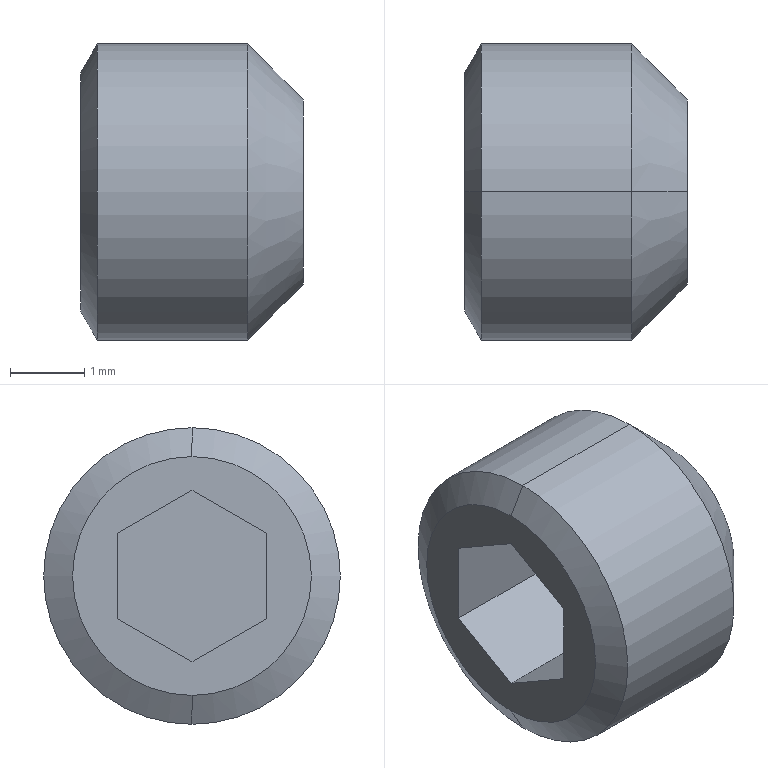Part | STEP file | socket set screw flat point_iso_ISO 4026 - M4 x 3-N | 1 solid | 15 faces | box 3 x 4 x 4 mm | volume 28.895 mm3 | plane 9 | cone 4 | cylinder 2 | commonest cylinder face diameters 4 x2
STEP:
#1=CARTESIAN_POINT('',(0.,0.,0.));
#2=DIRECTION('',(0.,0.,1.));
#3=DIRECTION('',(1.,0.,0.));
#4=AXIS2_PLACEMENT_3D('',#1,#2,#3);
#5=CARTESIAN_POINT('',(0.,0.,1.61));
#6=VERTEX_POINT('',#5);
#7=CARTESIAN_POINT('',(0.,0.,-1.61));
#8=VERTEX_POINT('',#7);
#9=CARTESIAN_POINT('',(0.,0.,0.));
#10=DIRECTION('',(-1.,0.,0.));
#11=DIRECTION('',(0.,0.,1.));
#12=AXIS2_PLACEMENT_3D('',#9,#10,#11);
#13=CIRCLE('',#12,1.61);
#14=CARTESIAN_POINT('',(0.,0.,0.));
#15=DIRECTION('',(1.,0.,0.));
#16=DIRECTION('',(0.,0.,-1.));
#17=AXIS2_PLACEMENT_3D('',#14,#15,#16);
#18=CONICAL_SURFACE('',#17,1.61,1.047);
#19=CARTESIAN_POINT('',(3.142,0.));
#20=DIRECTION('',(-1.,0.));
#21=VECTOR('',#20,1.);
#22=LINE('',#19,#21);
#23=(GEOMETRIC_REPRESENTATION_CONTEXT(2)PARAMETRIC_REPRESENTATION_CONTEXT()REPRESENTATION_CONTEXT('',''));
#24=DEFINITIONAL_REPRESENTATION('',(#22),#23);
#25=PCURVE('',#18,#24);
#26=CARTESIAN_POINT('',(0.,0.,0.));
#27=DIRECTION('',(-1.,0.,0.));
#28=DIRECTION('',(0.,0.,1.));
#29=AXIS2_PLACEMENT_3D('',#26,#27,#28);
#30=PLANE('',#29);
#31=CARTESIAN_POINT('',(0.,0.));
#32=DIRECTION('',(1.,0.));
#33=AXIS2_PLACEMENT_2D('',#31,#32);
#34=CIRCLE('',#33,1.61);
#35=(GEOMETRIC_REPRESENTATION_CONTEXT(2)PARAMETRIC_REPRESENTATION_CONTEXT()REPRESENTATION_CONTEXT('',''));
#36=DEFINITIONAL_REPRESENTATION('',(#34),#35);
#37=PCURVE('',#30,#36);
#38=SURFACE_CURVE('',#13,(#25,#37),.PCURVE_S1.);
#39=EDGE_CURVE('',#6,#8,#38,.T.);
#40=ORIENTED_EDGE('',*,*,#39,.F.);
#41=CARTESIAN_POINT('',(0.2252,0.,2.));
#42=VERTEX_POINT('',#41);
#43=CARTESIAN_POINT('',(0.,0.,1.61));
#44=DIRECTION('',(0.5,0.,0.866));
#45=VECTOR('',#44,1.);
#46=LINE('',#43,#45);
#47=CARTESIAN_POINT('',(3.142,0.));
#48=DIRECTION('',(0.,1.));
#49=VECTOR('',#48,1.);
#50=LINE('',#47,#49);
#51=(GEOMETRIC_REPRESENTATION_CONTEXT(2)PARAMETRIC_REPRESENTATION_CONTEXT()REPRESENTATION_CONTEXT('',''));
#52=DEFINITIONAL_REPRESENTATION('',(#50),#51);
#53=PCURVE('',#18,#52);
#54=CARTESIAN_POINT('',(0.,0.,0.));
#55=DIRECTION('',(1.,0.,0.));
#56=DIRECTION('',(0.,0.,-1.));
#57=AXIS2_PLACEMENT_3D('',#54,#55,#56);
#58=CONICAL_SURFACE('',#57,1.61,1.047);
#59=CARTESIAN_POINT('',(3.142,0.));
#60=DIRECTION('',(0.,1.));
#61=VECTOR('',#60,1.);
#62=LINE('',#59,#61);
#63=(GEOMETRIC_REPRESENTATION_CONTEXT(2)PARAMETRIC_REPRESENTATION_CONTEXT()REPRESENTATION_CONTEXT('',''));
#64=DEFINITIONAL_REPRESENTATION('',(#62),#63);
#65=PCURVE('',#58,#64);
#66=SURFACE_CURVE('',#46,(#53,#65),.PCURVE_S1.);
#67=EDGE_CURVE('',#6,#42,#66,.T.);
#68=ORIENTED_EDGE('',*,*,#67,.T.);
#69=CARTESIAN_POINT('',(0.2252,0.,-2.));
#70=VERTEX_POINT('',#69);
#71=CARTESIAN_POINT('',(0.2252,0.,0.));
#72=DIRECTION('',(-1.,0.,0.));
#73=DIRECTION('',(0.,0.,1.));
#74=AXIS2_PLACEMENT_3D('',#71,#72,#73);
#75=CIRCLE('',#74,2.);
#76=CARTESIAN_POINT('',(3.142,0.2252));
#77=DIRECTION('',(-1.,0.));
#78=VECTOR('',#77,1.);
#79=LINE('',#76,#78);
#80=(GEOMETRIC_REPRESENTATION_CONTEXT(2)PARAMETRIC_REPRESENTATION_CONTEXT()REPRESENTATION_CONTEXT('',''));
#81=DEFINITIONAL_REPRESENTATION('',(#79),#80);
#82=PCURVE('',#18,#81);
#83=CARTESIAN_POINT('',(-12.7,0.,0.));
#84=DIRECTION('',(-1.,0.,0.));
#85=DIRECTION('',(0.,0.,1.));
#86=AXIS2_PLACEMENT_3D('',#83,#84,#85);
#87=CYLINDRICAL_SURFACE('',#86,2.);
#88=CARTESIAN_POINT('',(0.,-12.925));
#89=DIRECTION('',(1.,0.));
#90=VECTOR('',#89,1.);
#91=LINE('',#88,#90);
#92=(GEOMETRIC_REPRESENTATION_CONTEXT(2)PARAMETRIC_REPRESENTATION_CONTEXT()REPRESENTATION_CONTEXT('',''));
#93=DEFINITIONAL_REPRESENTATION('',(#91),#92);
#94=PCURVE('',#87,#93);
#95=SURFACE_CURVE('',#75,(#82,#94),.PCURVE_S1.);
#96=EDGE_CURVE('',#42,#70,#95,.T.);
#97=ORIENTED_EDGE('',*,*,#96,.T.);
#98=CARTESIAN_POINT('',(0.,0.,-1.61));
#99=DIRECTION('',(0.5,0.,-0.866));
#100=VECTOR('',#99,1.);
#101=LINE('',#98,#100);
#102=CARTESIAN_POINT('',(0.,0.));
#103=DIRECTION('',(0.,1.));
#104=VECTOR('',#103,1.);
#105=LINE('',#102,#104);
#106=(GEOMETRIC_REPRESENTATION_CONTEXT(2)PARAMETRIC_REPRESENTATION_CONTEXT()REPRESENTATION_CONTEXT('',''));
#107=DEFINITIONAL_REPRESENTATION('',(#105),#106);
#108=PCURVE('',#18,#107);
#109=CARTESIAN_POINT('',(6.283,0.));
#110=DIRECTION('',(0.,1.));
#111=VECTOR('',#110,1.);
#112=LINE('',#109,#111);
#113=(GEOMETRIC_REPRESENTATION_CONTEXT(2)PARAMETRIC_REPRESENTATION_CONTEXT()REPRESENTATION_CONTEXT('',''));
#114=DEFINITIONAL_REPRESENTATION('',(#112),#113);
#115=PCURVE('',#58,#114);
#116=SURFACE_CURVE('',#101,(#108,#115),.PCURVE_S1.);
#117=EDGE_CURVE('',#8,#70,#116,.T.);
#118=ORIENTED_EDGE('',*,*,#117,.F.);
#119=EDGE_LOOP('',(#40,#68,#97,#118));
#120=FACE_BOUND('',#119,.T.);
#121=ADVANCED_FACE('',(#120),#18,.T.);
#122=CARTESIAN_POINT('',(2.25,0.,2.));
#123=VERTEX_POINT('',#122);
#124=CARTESIAN_POINT('',(2.25,0.,-2.));
#125=VERTEX_POINT('',#124);
#126=CARTESIAN_POINT('',(2.25,0.,0.));
#127=DIRECTION('',(-1.,0.,0.));
#128=DIRECTION('',(0.,0.,1.));
#129=AXIS2_PLACEMENT_3D('',#126,#127,#128);
#130=CIRCLE('',#129,2.);
#131=CARTESIAN_POINT('',(0.,-14.95));
#132=DIRECTION('',(1.,0.));
#133=VECTOR('',#132,1.);
#134=LINE('',#131,#133);
#135=(GEOMETRIC_REPRESENTATION_CONTEXT(2)PARAMETRIC_REPRESENTATION_CONTEXT()REPRESENTATION_CONTEXT('',''));
#136=DEFINITIONAL_REPRESENTATION('',(#134),#135);
#137=PCURVE('',#87,#136);
#138=CARTESIAN_POINT('',(2.25,0.,0.));
#139=DIRECTION('',(-1.,0.,0.));
#140=DIRECTION('',(0.,0.,1.));
#141=AXIS2_PLACEMENT_3D('',#138,#139,#140);
#142=CONICAL_SURFACE('',#141,2.,0.7854);
#143=CARTESIAN_POINT('',(0.,0.));
#144=DIRECTION('',(1.,0.));
#145=VECTOR('',#144,1.);
#146=LINE('',#143,#145);
#147=(GEOMETRIC_REPRESENTATION_CONTEXT(2)PARAMETRIC_REPRESENTATION_CONTEXT()REPRESENTATION_CONTEXT('',''));
#148=DEFINITIONAL_REPRESENTATION('',(#146),#147);
#149=PCURVE('',#142,#148);
#150=SURFACE_CURVE('',#130,(#137,#149),.PCURVE_S1.);
#151=EDGE_CURVE('',#123,#125,#150,.T.);
#152=ORIENTED_EDGE('',*,*,#151,.T.);
#153=CARTESIAN_POINT('',(-12.7,0.,-2.));
#154=DIRECTION('',(-1.,0.,0.));
#155=VECTOR('',#154,1.);
#156=LINE('',#153,#155);
#157=CARTESIAN_POINT('',(3.142,0.));
#158=DIRECTION('',(0.,1.));
#159=VECTOR('',#158,1.);
#160=LINE('',#157,#159);
#161=(GEOMETRIC_REPRESENTATION_CONTEXT(2)PARAMETRIC_REPRESENTATION_CONTEXT()REPRESENTATION_CONTEXT('',''));
#162=DEFINITIONAL_REPRESENTATION('',(#160),#161);
#163=PCURVE('',#87,#162);
#164=CARTESIAN_POINT('',(-12.7,0.,0.));
#165=DIRECTION('',(-1.,0.,0.));
#166=DIRECTION('',(0.,0.,1.));
#167=AXIS2_PLACEMENT_3D('',#164,#165,#166);
#168=CYLINDRICAL_SURFACE('',#167,2.);
#169=CARTESIAN_POINT('',(3.142,0.));
#170=DIRECTION('',(0.,1.));
#171=VECTOR('',#170,1.);
#172=LINE('',#169,#171);
#173=(GEOMETRIC_REPRESENTATION_CONTEXT(2)PARAMETRIC_REPRESENTATION_CONTEXT()REPRESENTATION_CONTEXT('',''));
#174=DEFINITIONAL_REPRESENTATION('',(#172),#173);
#175=PCURVE('',#168,#174);
#176=SURFACE_CURVE('',#156,(#163,#175),.PCURVE_S1.);
#177=EDGE_CURVE('',#125,#70,#176,.T.);
#178=ORIENTED_EDGE('',*,*,#177,.T.);
#179=ORIENTED_EDGE('',*,*,#96,.F.);
#180=CARTESIAN_POINT('',(-12.7,0.,2.));
#181=DIRECTION('',(-1.,0.,0.));
#182=VECTOR('',#181,1.);
#183=LINE('',#180,#182);
#184=CARTESIAN_POINT('',(0.,0.));
#185=DIRECTION('',(0.,1.));
#186=VECTOR('',#185,1.);
#187=LINE('',#184,#186);
#188=(GEOMETRIC_REPRESENTATION_CONTEXT(2)PARAMETRIC_REPRESENTATION_CONTEXT()REPRESENTATION_CONTEXT('',''));
#189=DEFINITIONAL_REPRESENTATION('',(#187),#188);
#190=PCURVE('',#87,#189);
#191=CARTESIAN_POINT('',(6.283,0.));
#192=DIRECTION('',(0.,1.));
#193=VECTOR('',#192,1.);
#194=LINE('',#191,#193);
#195=(GEOMETRIC_REPRESENTATION_CONTEXT(2)PARAMETRIC_REPRESENTATION_CONTEXT()REPRESENTATION_CONTEXT('',''));
#196=DEFINITIONAL_REPRESENTATION('',(#194),#195);
#197=PCURVE('',#168,#196);
#198=SURFACE_CURVE('',#183,(#190,#197),.PCURVE_S1.);
#199=EDGE_CURVE('',#123,#42,#198,.T.);
#200=ORIENTED_EDGE('',*,*,#199,.F.);
#201=EDGE_LOOP('',(#152,#178,#179,#200));
#202=FACE_BOUND('',#201,.T.);
#203=ADVANCED_FACE('',(#202),#87,.T.);
#204=CARTESIAN_POINT('',(3.,0.,1.25));
#205=VERTEX_POINT('',#204);
#206=CARTESIAN_POINT('',(3.,0.,-1.25));
#207=VERTEX_POINT('',#206);
#208=CARTESIAN_POINT('',(3.,0.,0.));
#209=DIRECTION('',(-1.,0.,0.));
#210=DIRECTION('',(0.,0.,1.));
#211=AXIS2_PLACEMENT_3D('',#208,#209,#210);
#212=CIRCLE('',#211,1.25);
#213=CARTESIAN_POINT('',(0.,-0.75));
#214=DIRECTION('',(1.,0.));
#215=VECTOR('',#214,1.);
#216=LINE('',#213,#215);
#217=(GEOMETRIC_REPRESENTATION_CONTEXT(2)PARAMETRIC_REPRESENTATION_CONTEXT()REPRESENTATION_CONTEXT('',''));
#218=DEFINITIONAL_REPRESENTATION('',(#216),#217);
#219=PCURVE('',#142,#218);
#220=CARTESIAN_POINT('',(3.,1.25,0.));
#221=DIRECTION('',(1.,0.,0.));
#222=DIRECTION('',(0.,0.,-1.));
#223=AXIS2_PLACEMENT_3D('',#220,#221,#222);
#224=PLANE('',#223);
#225=CARTESIAN_POINT('',(-1.25,-1.25));
#226=CARTESIAN_POINT('',(-1.25,0.9151));
#227=CARTESIAN_POINT('',(0.625,-0.1675));
#228=CARTESIAN_POINT('',(2.5,-1.25));
#229=CARTESIAN_POINT('',(0.625,-2.333));
#230=CARTESIAN_POINT('',(-1.25,-3.415));
#231=CARTESIAN_POINT('',(-1.25,-1.25));
#232=(BOUNDED_CURVE()B_SPLINE_CURVE(2,(#225,#226,#227,#228,#229,#230,#231),.UNSPECIFIED.,.T.,.F.)B_SPLINE_CURVE_WITH_KNOTS((1,2,2,2,2,1),(-2.094,0.,2.094,4.189,6.283,8.378),.UNSPECIFIED.)CURVE()GEOMETRIC_REPRESENTATION_ITEM()RATIONAL_B_SPLINE_CURVE((1.,0.5,1.,0.5,1.,0.5,1.))REPRESENTATION_ITEM(''));
#233=(GEOMETRIC_REPRESENTATION_CONTEXT(2)PARAMETRIC_REPRESENTATION_CONTEXT()REPRESENTATION_CONTEXT('',''));
#234=DEFINITIONAL_REPRESENTATION('',(#232),#233);
#235=PCURVE('',#224,#234);
#236=SURFACE_CURVE('',#212,(#219,#235),.PCURVE_S1.);
#237=EDGE_CURVE('',#205,#207,#236,.T.);
#238=ORIENTED_EDGE('',*,*,#237,.T.);
#239=CARTESIAN_POINT('',(2.25,0.,-2.));
#240=DIRECTION('',(-0.7071,0.,-0.7071));
#241=VECTOR('',#240,1.);
#242=LINE('',#239,#241);
#243=CARTESIAN_POINT('',(3.142,0.));
#244=DIRECTION('',(0.,1.));
#245=VECTOR('',#244,1.);
#246=LINE('',#243,#245);
#247=(GEOMETRIC_REPRESENTATION_CONTEXT(2)PARAMETRIC_REPRESENTATION_CONTEXT()REPRESENTATION_CONTEXT('',''));
#248=DEFINITIONAL_REPRESENTATION('',(#246),#247);
#249=PCURVE('',#142,#248);
#250=CARTESIAN_POINT('',(2.25,0.,0.));
#251=DIRECTION('',(-1.,0.,0.));
#252=DIRECTION('',(0.,0.,1.));
#253=AXIS2_PLACEMENT_3D('',#250,#251,#252);
#254=CONICAL_SURFACE('',#253,2.,0.7854);
#255=CARTESIAN_POINT('',(3.142,0.));
#256=DIRECTION('',(0.,1.));
#257=VECTOR('',#256,1.);
#258=LINE('',#255,#257);
#259=(GEOMETRIC_REPRESENTATION_CONTEXT(2)PARAMETRIC_REPRESENTATION_CONTEXT()REPRESENTATION_CONTEXT('',''));
#260=DEFINITIONAL_REPRESENTATION('',(#258),#259);
#261=PCURVE('',#254,#260);
#262=SURFACE_CURVE('',#242,(#249,#261),.PCURVE_S1.);
#263=EDGE_CURVE('',#207,#125,#262,.T.);
#264=ORIENTED_EDGE('',*,*,#263,.T.);
#265=ORIENTED_EDGE('',*,*,#151,.F.);
#266=CARTESIAN_POINT('',(2.25,0.,2.));
#267=DIRECTION('',(-0.7071,0.,0.7071));
#268=VECTOR('',#267,1.);
#269=LINE('',#266,#268);
#270=CARTESIAN_POINT('',(0.,0.));
#271=DIRECTION('',(0.,1.));
#272=VECTOR('',#271,1.);
#273=LINE('',#270,#272);
#274=(GEOMETRIC_REPRESENTATION_CONTEXT(2)PARAMETRIC_REPRESENTATION_CONTEXT()REPRESENTATION_CONTEXT('',''));
#275=DEFINITIONAL_REPRESENTATION('',(#273),#274);
#276=PCURVE('',#142,#275);
#277=CARTESIAN_POINT('',(6.283,0.));
#278=DIRECTION('',(0.,1.));
#279=VECTOR('',#278,1.);
#280=LINE('',#277,#279);
#281=(GEOMETRIC_REPRESENTATION_CONTEXT(2)PARAMETRIC_REPRESENTATION_CONTEXT()REPRESENTATION_CONTEXT('',''));
#282=DEFINITIONAL_REPRESENTATION('',(#280),#281);
#283=PCURVE('',#254,#282);
#284=SURFACE_CURVE('',#269,(#276,#283),.PCURVE_S1.);
#285=EDGE_CURVE('',#205,#123,#284,.T.);
#286=ORIENTED_EDGE('',*,*,#285,.F.);
#287=EDGE_LOOP('',(#238,#264,#265,#286));
#288=FACE_BOUND('',#287,.T.);
#289=ADVANCED_FACE('',(#288),#142,.T.);
#290=CARTESIAN_POINT('',(0.,0.,0.));
#291=DIRECTION('',(-1.,0.,0.));
#292=DIRECTION('',(0.,0.,1.));
#293=AXIS2_PLACEMENT_3D('',#290,#291,#292);
#294=CIRCLE('',#293,1.61);
#295=CARTESIAN_POINT('',(0.,0.));
#296=DIRECTION('',(1.,0.));
#297=AXIS2_PLACEMENT_2D('',#295,#296);
#298=CIRCLE('',#297,1.61);
#299=(GEOMETRIC_REPRESENTATION_CONTEXT(2)PARAMETRIC_REPRESENTATION_CONTEXT()REPRESENTATION_CONTEXT('',''));
#300=DEFINITIONAL_REPRESENTATION('',(#298),#299);
#301=PCURVE('',#30,#300);
#302=CARTESIAN_POINT('',(9.425,0.));
#303=DIRECTION('',(-1.,0.));
#304=VECTOR('',#303,1.);
#305=LINE('',#302,#304);
#306=(GEOMETRIC_REPRESENTATION_CONTEXT(2)PARAMETRIC_REPRESENTATION_CONTEXT()REPRESENTATION_CONTEXT('',''));
#307=DEFINITIONAL_REPRESENTATION('',(#305),#306);
#308=PCURVE('',#58,#307);
#309=SURFACE_CURVE('',#294,(#301,#308),.PCURVE_S1.);
#310=EDGE_CURVE('',#8,#6,#309,.T.);
#311=ORIENTED_EDGE('',*,*,#310,.T.);
#312=ORIENTED_EDGE('',*,*,#39,.T.);
#313=EDGE_LOOP('',(#311,#312));
#314=FACE_BOUND('',#313,.T.);
#315=CARTESIAN_POINT('',(0.,1.,0.5774));
#316=VERTEX_POINT('',#315);
#317=CARTESIAN_POINT('',(0.,1.,-0.5774));
#318=VERTEX_POINT('',#317);
#319=CARTESIAN_POINT('',(0.,1.,0.5774));
#320=DIRECTION('',(0.,0.,-1.));
#321=VECTOR('',#320,1.);
#322=LINE('',#319,#321);
#323=CARTESIAN_POINT('',(0.5774,1.));
#324=DIRECTION('',(-1.,0.));
#325=VECTOR('',#324,1.);
#326=LINE('',#323,#325);
#327=(GEOMETRIC_REPRESENTATION_CONTEXT(2)PARAMETRIC_REPRESENTATION_CONTEXT()REPRESENTATION_CONTEXT('',''));
#328=DEFINITIONAL_REPRESENTATION('',(#326),#327);
#329=PCURVE('',#30,#328);
#330=CARTESIAN_POINT('',(1.5,1.,0.5774));
#331=DIRECTION('',(0.,1.,0.));
#332=DIRECTION('',(0.,0.,1.));
#333=AXIS2_PLACEMENT_3D('',#330,#331,#332);
#334=PLANE('',#333);
#335=CARTESIAN_POINT('',(0.,-1.5));
#336=DIRECTION('',(-1.,0.));
#337=VECTOR('',#336,1.);
#338=LINE('',#335,#337);
#339=(GEOMETRIC_REPRESENTATION_CONTEXT(2)PARAMETRIC_REPRESENTATION_CONTEXT()REPRESENTATION_CONTEXT('',''));
#340=DEFINITIONAL_REPRESENTATION('',(#338),#339);
#341=PCURVE('',#334,#340);
#342=SURFACE_CURVE('',#322,(#329,#341),.PCURVE_S1.);
#343=EDGE_CURVE('',#316,#318,#342,.T.);
#344=ORIENTED_EDGE('',*,*,#343,.F.);
#345=CARTESIAN_POINT('',(0.,0.,1.155));
#346=VERTEX_POINT('',#345);
#347=CARTESIAN_POINT('',(0.,1.,0.5774));
#348=DIRECTION('',(0.,-0.866,0.5));
#349=VECTOR('',#348,1.);
#350=LINE('',#347,#349);
#351=CARTESIAN_POINT('',(0.5774,1.));
#352=DIRECTION('',(0.5,-0.866));
#353=VECTOR('',#352,1.);
#354=LINE('',#351,#353);
#355=(GEOMETRIC_REPRESENTATION_CONTEXT(2)PARAMETRIC_REPRESENTATION_CONTEXT()REPRESENTATION_CONTEXT('',''));
#356=DEFINITIONAL_REPRESENTATION('',(#354),#355);
#357=PCURVE('',#30,#356);
#358=CARTESIAN_POINT('',(1.5,1.,0.5774));
#359=DIRECTION('',(0.,-0.5,-0.866));
#360=DIRECTION('',(0.,0.866,-0.5));
#361=AXIS2_PLACEMENT_3D('',#358,#359,#360);
#362=PLANE('',#361);
#363=CARTESIAN_POINT('',(0.,-1.5));
#364=DIRECTION('',(-1.,0.));
#365=VECTOR('',#364,1.);
#366=LINE('',#363,#365);
#367=(GEOMETRIC_REPRESENTATION_CONTEXT(2)PARAMETRIC_REPRESENTATION_CONTEXT()REPRESENTATION_CONTEXT('',''));
#368=DEFINITIONAL_REPRESENTATION('',(#366),#367);
#369=PCURVE('',#362,#368);
#370=SURFACE_CURVE('',#350,(#357,#369),.PCURVE_S1.);
#371=EDGE_CURVE('',#316,#346,#370,.T.);
#372=ORIENTED_EDGE('',*,*,#371,.T.);
#373=CARTESIAN_POINT('',(0.,-1.,0.5774));
#374=VERTEX_POINT('',#373);
#375=CARTESIAN_POINT('',(0.,-1.,0.5774));
#376=DIRECTION('',(0.,0.866,0.5));
#377=VECTOR('',#376,1.);
#378=LINE('',#375,#377);
#379=CARTESIAN_POINT('',(0.5774,-1.));
#380=DIRECTION('',(0.5,0.866));
#381=VECTOR('',#380,1.);
#382=LINE('',#379,#381);
#383=(GEOMETRIC_REPRESENTATION_CONTEXT(2)PARAMETRIC_REPRESENTATION_CONTEXT()REPRESENTATION_CONTEXT('',''));
#384=DEFINITIONAL_REPRESENTATION('',(#382),#383);
#385=PCURVE('',#30,#384);
#386=CARTESIAN_POINT('',(1.5,-1.,0.5774));
#387=DIRECTION('',(0.,-0.5,0.866));
#388=DIRECTION('',(0.,-0.866,-0.5));
#389=AXIS2_PLACEMENT_3D('',#386,#387,#388);
#390=PLANE('',#389);
#391=CARTESIAN_POINT('',(0.,-1.5));
#392=DIRECTION('',(-1.,0.));
#393=VECTOR('',#392,1.);
#394=LINE('',#391,#393);
#395=(GEOMETRIC_REPRESENTATION_CONTEXT(2)PARAMETRIC_REPRESENTATION_CONTEXT()REPRESENTATION_CONTEXT('',''));
#396=DEFINITIONAL_REPRESENTATION('',(#394),#395);
#397=PCURVE('',#390,#396);
#398=SURFACE_CURVE('',#378,(#385,#397),.PCURVE_S1.);
#399=EDGE_CURVE('',#374,#346,#398,.T.);
#400=ORIENTED_EDGE('',*,*,#399,.F.);
#401=CARTESIAN_POINT('',(0.,-1.,-0.5774));
#402=VERTEX_POINT('',#401);
#403=CARTESIAN_POINT('',(0.,-1.,0.5774));
#404=DIRECTION('',(0.,0.,-1.));
#405=VECTOR('',#404,1.);
#406=LINE('',#403,#405);
#407=CARTESIAN_POINT('',(0.5774,-1.));
#408=DIRECTION('',(-1.,0.));
#409=VECTOR('',#408,1.);
#410=LINE('',#407,#409);
#411=(GEOMETRIC_REPRESENTATION_CONTEXT(2)PARAMETRIC_REPRESENTATION_CONTEXT()REPRESENTATION_CONTEXT('',''));
#412=DEFINITIONAL_REPRESENTATION('',(#410),#411);
#413=PCURVE('',#30,#412);
#414=CARTESIAN_POINT('',(1.5,-1.,0.5774));
#415=DIRECTION('',(0.,1.,0.));
#416=DIRECTION('',(0.,0.,1.));
#417=AXIS2_PLACEMENT_3D('',#414,#415,#416);
#418=PLANE('',#417);
#419=CARTESIAN_POINT('',(0.,-1.5));
#420=DIRECTION('',(-1.,0.));
#421=VECTOR('',#420,1.);
#422=LINE('',#419,#421);
#423=(GEOMETRIC_REPRESENTATION_CONTEXT(2)PARAMETRIC_REPRESENTATION_CONTEXT()REPRESENTATION_CONTEXT('',''));
#424=DEFINITIONAL_REPRESENTATION('',(#422),#423);
#425=PCURVE('',#418,#424);
#426=SURFACE_CURVE('',#406,(#413,#425),.PCURVE_S1.);
#427=EDGE_CURVE('',#374,#402,#426,.T.);
#428=ORIENTED_EDGE('',*,*,#427,.T.);
#429=CARTESIAN_POINT('',(0.,0.,-1.155));
#430=VERTEX_POINT('',#429);
#431=CARTESIAN_POINT('',(0.,-1.,-0.5774));
#432=DIRECTION('',(0.,0.866,-0.5));
#433=VECTOR('',#432,1.);
#434=LINE('',#431,#433);
#435=CARTESIAN_POINT('',(-0.5774,-1.));
#436=DIRECTION('',(-0.5,0.866));
#437=VECTOR('',#436,1.);
#438=LINE('',#435,#437);
#439=(GEOMETRIC_REPRESENTATION_CONTEXT(2)PARAMETRIC_REPRESENTATION_CONTEXT()REPRESENTATION_CONTEXT('',''));
#440=DEFINITIONAL_REPRESENTATION('',(#438),#439);
#441=PCURVE('',#30,#440);
#442=CARTESIAN_POINT('',(1.5,-1.,-0.5774));
#443=DIRECTION('',(0.,0.5,0.866));
#444=DIRECTION('',(0.,-0.866,0.5));
#445=AXIS2_PLACEMENT_3D('',#442,#443,#444);
#446=PLANE('',#445);
#447=CARTESIAN_POINT('',(0.,-1.5));
#448=DIRECTION('',(-1.,0.));
#449=VECTOR('',#448,1.);
#450=LINE('',#447,#449);
#451=(GEOMETRIC_REPRESENTATION_CONTEXT(2)PARAMETRIC_REPRESENTATION_CONTEXT()REPRESENTATION_CONTEXT('',''));
#452=DEFINITIONAL_REPRESENTATION('',(#450),#451);
#453=PCURVE('',#446,#452);
#454=SURFACE_CURVE('',#434,(#441,#453),.PCURVE_S1.);
#455=EDGE_CURVE('',#402,#430,#454,.T.);
#456=ORIENTED_EDGE('',*,*,#455,.T.);
#457=CARTESIAN_POINT('',(0.,1.,-0.5774));
#458=DIRECTION('',(0.,-0.866,-0.5));
#459=VECTOR('',#458,1.);
#460=LINE('',#457,#459);
#461=CARTESIAN_POINT('',(-0.5774,1.));
#462=DIRECTION('',(-0.5,-0.866));
#463=VECTOR('',#462,1.);
#464=LINE('',#461,#463);
#465=(GEOMETRIC_REPRESENTATION_CONTEXT(2)PARAMETRIC_REPRESENTATION_CONTEXT()REPRESENTATION_CONTEXT('',''));
#466=DEFINITIONAL_REPRESENTATION('',(#464),#465);
#467=PCURVE('',#30,#466);
#468=CARTESIAN_POINT('',(1.5,1.,-0.5774));
#469=DIRECTION('',(0.,0.5,-0.866));
#470=DIRECTION('',(0.,0.866,0.5));
#471=AXIS2_PLACEMENT_3D('',#468,#469,#470);
#472=PLANE('',#471);
#473=CARTESIAN_POINT('',(0.,-1.5));
#474=DIRECTION('',(-1.,0.));
#475=VECTOR('',#474,1.);
#476=LINE('',#473,#475);
#477=(GEOMETRIC_REPRESENTATION_CONTEXT(2)PARAMETRIC_REPRESENTATION_CONTEXT()REPRESENTATION_CONTEXT('',''));
#478=DEFINITIONAL_REPRESENTATION('',(#476),#477);
#479=PCURVE('',#472,#478);
#480=SURFACE_CURVE('',#460,(#467,#479),.PCURVE_S1.);
#481=EDGE_CURVE('',#318,#430,#480,.T.);
#482=ORIENTED_EDGE('',*,*,#481,.F.);
#483=EDGE_LOOP('',(#344,#372,#400,#428,#456,#482));
#484=FACE_BOUND('',#483,.T.);
#485=ADVANCED_FACE('',(#314,#484),#30,.T.);
#486=ORIENTED_EDGE('',*,*,#237,.F.);
#487=CARTESIAN_POINT('',(3.,0.,0.));
#488=DIRECTION('',(-1.,0.,0.));
#489=DIRECTION('',(0.,0.,1.));
#490=AXIS2_PLACEMENT_3D('',#487,#488,#489);
#491=CIRCLE('',#490,1.25);
#492=CARTESIAN_POINT('',(-1.25,-1.25));
#493=CARTESIAN_POINT('',(-1.25,0.9151));
#494=CARTESIAN_POINT('',(0.625,-0.1675));
#495=CARTESIAN_POINT('',(2.5,-1.25));
#496=CARTESIAN_POINT('',(0.625,-2.333));
#497=CARTESIAN_POINT('',(-1.25,-3.415));
#498=CARTESIAN_POINT('',(-1.25,-1.25));
#499=(BOUNDED_CURVE()B_SPLINE_CURVE(2,(#492,#493,#494,#495,#496,#497,#498),.UNSPECIFIED.,.T.,.F.)B_SPLINE_CURVE_WITH_KNOTS((1,2,2,2,2,1),(-2.094,0.,2.094,4.189,6.283,8.378),.UNSPECIFIED.)CURVE()GEOMETRIC_REPRESENTATION_ITEM()RATIONAL_B_SPLINE_CURVE((1.,0.5,1.,0.5,1.,0.5,1.))REPRESENTATION_ITEM(''));
#500=(GEOMETRIC_REPRESENTATION_CONTEXT(2)PARAMETRIC_REPRESENTATION_CONTEXT()REPRESENTATION_CONTEXT('',''));
#501=DEFINITIONAL_REPRESENTATION('',(#499),#500);
#502=PCURVE('',#224,#501);
#503=CARTESIAN_POINT('',(0.,-0.75));
#504=DIRECTION('',(1.,0.));
#505=VECTOR('',#504,1.);
#506=LINE('',#503,#505);
#507=(GEOMETRIC_REPRESENTATION_CONTEXT(2)PARAMETRIC_REPRESENTATION_CONTEXT()REPRESENTATION_CONTEXT('',''));
#508=DEFINITIONAL_REPRESENTATION('',(#506),#507);
#509=PCURVE('',#254,#508);
#510=SURFACE_CURVE('',#491,(#502,#509),.PCURVE_S1.);
#511=EDGE_CURVE('',#207,#205,#510,.T.);
#512=ORIENTED_EDGE('',*,*,#511,.F.);
#513=EDGE_LOOP('',(#486,#512));
#514=FACE_BOUND('',#513,.T.);
#515=ADVANCED_FACE('',(#514),#224,.T.);
#516=ORIENTED_EDGE('',*,*,#263,.F.);
#517=ORIENTED_EDGE('',*,*,#511,.T.);
#518=ORIENTED_EDGE('',*,*,#285,.T.);
#519=CARTESIAN_POINT('',(2.25,0.,0.));
#520=DIRECTION('',(-1.,0.,0.));
#521=DIRECTION('',(0.,0.,1.));
#522=AXIS2_PLACEMENT_3D('',#519,#520,#521);
#523=CIRCLE('',#522,2.);
#524=CARTESIAN_POINT('',(0.,0.));
#525=DIRECTION('',(1.,0.));
#526=VECTOR('',#525,1.);
#527=LINE('',#524,#526);
#528=(GEOMETRIC_REPRESENTATION_CONTEXT(2)PARAMETRIC_REPRESENTATION_CONTEXT()REPRESENTATION_CONTEXT('',''));
#529=DEFINITIONAL_REPRESENTATION('',(#527),#528);
#530=PCURVE('',#254,#529);
#531=CARTESIAN_POINT('',(0.,-14.95));
#532=DIRECTION('',(1.,0.));
#533=VECTOR('',#532,1.);
#534=LINE('',#531,#533);
#535=(GEOMETRIC_REPRESENTATION_CONTEXT(2)PARAMETRIC_REPRESENTATION_CONTEXT()REPRESENTATION_CONTEXT('',''));
#536=DEFINITIONAL_REPRESENTATION('',(#534),#535);
#537=PCURVE('',#168,#536);
#538=SURFACE_CURVE('',#523,(#530,#537),.PCURVE_S1.);
#539=EDGE_CURVE('',#125,#123,#538,.T.);
#540=ORIENTED_EDGE('',*,*,#539,.F.);
#541=EDGE_LOOP('',(#516,#517,#518,#540));
#542=FACE_BOUND('',#541,.T.);
#543=ADVANCED_FACE('',(#542),#254,.T.);
#544=ORIENTED_EDGE('',*,*,#177,.F.);
#545=ORIENTED_EDGE('',*,*,#539,.T.);
#546=ORIENTED_EDGE('',*,*,#199,.T.);
#547=CARTESIAN_POINT('',(0.2252,0.,0.));
#548=DIRECTION('',(-1.,0.,0.));
#549=DIRECTION('',(0.,0.,1.));
#550=AXIS2_PLACEMENT_3D('',#547,#548,#549);
#551=CIRCLE('',#550,2.);
#552=CARTESIAN_POINT('',(0.,-12.925));
#553=DIRECTION('',(1.,0.));
#554=VECTOR('',#553,1.);
#555=LINE('',#552,#554);
#556=(GEOMETRIC_REPRESENTATION_CONTEXT(2)PARAMETRIC_REPRESENTATION_CONTEXT()REPRESENTATION_CONTEXT('',''));
#557=DEFINITIONAL_REPRESENTATION('',(#555),#556);
#558=PCURVE('',#168,#557);
#559=CARTESIAN_POINT('',(9.425,0.2252));
#560=DIRECTION('',(-1.,0.));
#561=VECTOR('',#560,1.);
#562=LINE('',#559,#561);
#563=(GEOMETRIC_REPRESENTATION_CONTEXT(2)PARAMETRIC_REPRESENTATION_CONTEXT()REPRESENTATION_CONTEXT('',''));
#564=DEFINITIONAL_REPRESENTATION('',(#562),#563);
#565=PCURVE('',#58,#564);
#566=SURFACE_CURVE('',#551,(#558,#565),.PCURVE_S1.);
#567=EDGE_CURVE('',#70,#42,#566,.T.);
#568=ORIENTED_EDGE('',*,*,#567,.F.);
#569=EDGE_LOOP('',(#544,#545,#546,#568));
#570=FACE_BOUND('',#569,.T.);
#571=ADVANCED_FACE('',(#570),#168,.T.);
#572=ORIENTED_EDGE('',*,*,#67,.F.);
#573=ORIENTED_EDGE('',*,*,#310,.F.);
#574=ORIENTED_EDGE('',*,*,#117,.T.);
#575=ORIENTED_EDGE('',*,*,#567,.T.);
#576=EDGE_LOOP('',(#572,#573,#574,#575));
#577=FACE_BOUND('',#576,.T.);
#578=ADVANCED_FACE('',(#577),#58,.T.);
#579=ORIENTED_EDGE('',*,*,#371,.F.);
#580=CARTESIAN_POINT('',(1.5,1.,0.5774));
#581=VERTEX_POINT('',#580);
#582=CARTESIAN_POINT('',(1.5,1.,0.5774));
#583=DIRECTION('',(-1.,0.,0.));
#584=VECTOR('',#583,1.);
#585=LINE('',#582,#584);
#586=CARTESIAN_POINT('',(0.,0.));
#587=DIRECTION('',(0.,-1.));
#588=VECTOR('',#587,1.);
#589=LINE('',#586,#588);
#590=(GEOMETRIC_REPRESENTATION_CONTEXT(2)PARAMETRIC_REPRESENTATION_CONTEXT()REPRESENTATION_CONTEXT('',''));
#591=DEFINITIONAL_REPRESENTATION('',(#589),#590);
#592=PCURVE('',#362,#591);
#593=CARTESIAN_POINT('',(0.,0.));
#594=DIRECTION('',(0.,-1.));
#595=VECTOR('',#594,1.);
#596=LINE('',#593,#595);
#597=(GEOMETRIC_REPRESENTATION_CONTEXT(2)PARAMETRIC_REPRESENTATION_CONTEXT()REPRESENTATION_CONTEXT('',''));
#598=DEFINITIONAL_REPRESENTATION('',(#596),#597);
#599=PCURVE('',#334,#598);
#600=SURFACE_CURVE('',#585,(#592,#599),.PCURVE_S1.);
#601=EDGE_CURVE('',#581,#316,#600,.T.);
#602=ORIENTED_EDGE('',*,*,#601,.F.);
#603=CARTESIAN_POINT('',(1.5,0.,1.155));
#604=VERTEX_POINT('',#603);
#605=CARTESIAN_POINT('',(1.5,1.,0.5774));
#606=DIRECTION('',(0.,-0.866,0.5));
#607=VECTOR('',#606,1.);
#608=LINE('',#605,#607);
#609=CARTESIAN_POINT('',(0.,0.));
#610=DIRECTION('',(-1.,0.));
#611=VECTOR('',#610,1.);
#612=LINE('',#609,#611);
#613=(GEOMETRIC_REPRESENTATION_CONTEXT(2)PARAMETRIC_REPRESENTATION_CONTEXT()REPRESENTATION_CONTEXT('',''));
#614=DEFINITIONAL_REPRESENTATION('',(#612),#613);
#615=PCURVE('',#362,#614);
#616=CARTESIAN_POINT('',(1.5,0.,1.155));
#617=DIRECTION('',(-1.,0.,0.));
#618=DIRECTION('',(0.,0.,1.));
#619=AXIS2_PLACEMENT_3D('',#616,#617,#618);
#620=PLANE('',#619);
#621=CARTESIAN_POINT('',(-0.5774,1.));
#622=DIRECTION('',(0.5,-0.866));
#623=VECTOR('',#622,1.);
#624=LINE('',#621,#623);
#625=(GEOMETRIC_REPRESENTATION_CONTEXT(2)PARAMETRIC_REPRESENTATION_CONTEXT()REPRESENTATION_CONTEXT('',''));
#626=DEFINITIONAL_REPRESENTATION('',(#624),#625);
#627=PCURVE('',#620,#626);
#628=SURFACE_CURVE('',#608,(#615,#627),.PCURVE_S1.);
#629=EDGE_CURVE('',#581,#604,#628,.T.);
#630=ORIENTED_EDGE('',*,*,#629,.T.);
#631=CARTESIAN_POINT('',(1.5,0.,1.155));
#632=DIRECTION('',(-1.,0.,0.));
#633=VECTOR('',#632,1.);
#634=LINE('',#631,#633);
#635=CARTESIAN_POINT('',(-1.155,0.));
#636=DIRECTION('',(0.,-1.));
#637=VECTOR('',#636,1.);
#638=LINE('',#635,#637);
#639=(GEOMETRIC_REPRESENTATION_CONTEXT(2)PARAMETRIC_REPRESENTATION_CONTEXT()REPRESENTATION_CONTEXT('',''));
#640=DEFINITIONAL_REPRESENTATION('',(#638),#639);
#641=PCURVE('',#362,#640);
#642=CARTESIAN_POINT('',(-1.155,0.));
#643=DIRECTION('',(0.,-1.));
#644=VECTOR('',#643,1.);
#645=LINE('',#642,#644);
#646=(GEOMETRIC_REPRESENTATION_CONTEXT(2)PARAMETRIC_REPRESENTATION_CONTEXT()REPRESENTATION_CONTEXT('',''));
#647=DEFINITIONAL_REPRESENTATION('',(#645),#646);
#648=PCURVE('',#390,#647);
#649=SURFACE_CURVE('',#634,(#641,#648),.PCURVE_S1.);
#650=EDGE_CURVE('',#604,#346,#649,.T.);
#651=ORIENTED_EDGE('',*,*,#650,.T.);
#652=EDGE_LOOP('',(#579,#602,#630,#651));
#653=FACE_BOUND('',#652,.T.);
#654=ADVANCED_FACE('',(#653),#362,.T.);
#655=ORIENTED_EDGE('',*,*,#399,.T.);
#656=ORIENTED_EDGE('',*,*,#650,.F.);
#657=CARTESIAN_POINT('',(1.5,-1.,0.5774));
#658=VERTEX_POINT('',#657);
#659=CARTESIAN_POINT('',(1.5,-1.,0.5774));
#660=DIRECTION('',(0.,0.866,0.5));
#661=VECTOR('',#660,1.);
#662=LINE('',#659,#661);
#663=CARTESIAN_POINT('',(0.,0.));
#664=DIRECTION('',(-1.,0.));
#665=VECTOR('',#664,1.);
#666=LINE('',#663,#665);
#667=(GEOMETRIC_REPRESENTATION_CONTEXT(2)PARAMETRIC_REPRESENTATION_CONTEXT()REPRESENTATION_CONTEXT('',''));
#668=DEFINITIONAL_REPRESENTATION('',(#666),#667);
#669=PCURVE('',#390,#668);
#670=CARTESIAN_POINT('',(-0.5774,-1.));
#671=DIRECTION('',(0.5,0.866));
#672=VECTOR('',#671,1.);
#673=LINE('',#670,#672);
#674=(GEOMETRIC_REPRESENTATION_CONTEXT(2)PARAMETRIC_REPRESENTATION_CONTEXT()REPRESENTATION_CONTEXT('',''));
#675=DEFINITIONAL_REPRESENTATION('',(#673),#674);
#676=PCURVE('',#620,#675);
#677=SURFACE_CURVE('',#662,(#669,#676),.PCURVE_S1.);
#678=EDGE_CURVE('',#658,#604,#677,.T.);
#679=ORIENTED_EDGE('',*,*,#678,.F.);
#680=CARTESIAN_POINT('',(1.5,-1.,0.5774));
#681=DIRECTION('',(-1.,0.,0.));
#682=VECTOR('',#681,1.);
#683=LINE('',#680,#682);
#684=CARTESIAN_POINT('',(0.,0.));
#685=DIRECTION('',(0.,-1.));
#686=VECTOR('',#685,1.);
#687=LINE('',#684,#686);
#688=(GEOMETRIC_REPRESENTATION_CONTEXT(2)PARAMETRIC_REPRESENTATION_CONTEXT()REPRESENTATION_CONTEXT('',''));
#689=DEFINITIONAL_REPRESENTATION('',(#687),#688);
#690=PCURVE('',#390,#689);
#691=CARTESIAN_POINT('',(0.,0.));
#692=DIRECTION('',(0.,-1.));
#693=VECTOR('',#692,1.);
#694=LINE('',#691,#693);
#695=(GEOMETRIC_REPRESENTATION_CONTEXT(2)PARAMETRIC_REPRESENTATION_CONTEXT()REPRESENTATION_CONTEXT('',''));
#696=DEFINITIONAL_REPRESENTATION('',(#694),#695);
#697=PCURVE('',#418,#696);
#698=SURFACE_CURVE('',#683,(#690,#697),.PCURVE_S1.);
#699=EDGE_CURVE('',#658,#374,#698,.T.);
#700=ORIENTED_EDGE('',*,*,#699,.T.);
#701=EDGE_LOOP('',(#655,#656,#679,#700));
#702=FACE_BOUND('',#701,.T.);
#703=ADVANCED_FACE('',(#702),#390,.F.);
#704=ORIENTED_EDGE('',*,*,#427,.F.);
#705=ORIENTED_EDGE('',*,*,#699,.F.);
#706=CARTESIAN_POINT('',(1.5,-1.,-0.5774));
#707=VERTEX_POINT('',#706);
#708=CARTESIAN_POINT('',(1.5,-1.,0.5774));
#709=DIRECTION('',(0.,0.,-1.));
#710=VECTOR('',#709,1.);
#711=LINE('',#708,#710);
#712=CARTESIAN_POINT('',(0.,0.));
#713=DIRECTION('',(-1.,0.));
#714=VECTOR('',#713,1.);
#715=LINE('',#712,#714);
#716=(GEOMETRIC_REPRESENTATION_CONTEXT(2)PARAMETRIC_REPRESENTATION_CONTEXT()REPRESENTATION_CONTEXT('',''));
#717=DEFINITIONAL_REPRESENTATION('',(#715),#716);
#718=PCURVE('',#418,#717);
#719=CARTESIAN_POINT('',(-0.5774,-1.));
#720=DIRECTION('',(-1.,0.));
#721=VECTOR('',#720,1.);
#722=LINE('',#719,#721);
#723=(GEOMETRIC_REPRESENTATION_CONTEXT(2)PARAMETRIC_REPRESENTATION_CONTEXT()REPRESENTATION_CONTEXT('',''));
#724=DEFINITIONAL_REPRESENTATION('',(#722),#723);
#725=PCURVE('',#620,#724);
#726=SURFACE_CURVE('',#711,(#718,#725),.PCURVE_S1.);
#727=EDGE_CURVE('',#658,#707,#726,.T.);
#728=ORIENTED_EDGE('',*,*,#727,.T.);
#729=CARTESIAN_POINT('',(1.5,-1.,-0.5774));
#730=DIRECTION('',(-1.,0.,0.));
#731=VECTOR('',#730,1.);
#732=LINE('',#729,#731);
#733=CARTESIAN_POINT('',(-1.155,0.));
#734=DIRECTION('',(0.,-1.));
#735=VECTOR('',#734,1.);
#736=LINE('',#733,#735);
#737=(GEOMETRIC_REPRESENTATION_CONTEXT(2)PARAMETRIC_REPRESENTATION_CONTEXT()REPRESENTATION_CONTEXT('',''));
#738=DEFINITIONAL_REPRESENTATION('',(#736),#737);
#739=PCURVE('',#418,#738);
#740=CARTESIAN_POINT('',(0.,0.));
#741=DIRECTION('',(0.,-1.));
#742=VECTOR('',#741,1.);
#743=LINE('',#740,#742);
#744=(GEOMETRIC_REPRESENTATION_CONTEXT(2)PARAMETRIC_REPRESENTATION_CONTEXT()REPRESENTATION_CONTEXT('',''));
#745=DEFINITIONAL_REPRESENTATION('',(#743),#744);
#746=PCURVE('',#446,#745);
#747=SURFACE_CURVE('',#732,(#739,#746),.PCURVE_S1.);
#748=EDGE_CURVE('',#707,#402,#747,.T.);
#749=ORIENTED_EDGE('',*,*,#748,.T.);
#750=EDGE_LOOP('',(#704,#705,#728,#749));
#751=FACE_BOUND('',#750,.T.);
#752=ADVANCED_FACE('',(#751),#418,.T.);
#753=ORIENTED_EDGE('',*,*,#455,.F.);
#754=ORIENTED_EDGE('',*,*,#748,.F.);
#755=CARTESIAN_POINT('',(1.5,0.,-1.155));
#756=VERTEX_POINT('',#755);
#757=CARTESIAN_POINT('',(1.5,-1.,-0.5774));
#758=DIRECTION('',(0.,0.866,-0.5));
#759=VECTOR('',#758,1.);
#760=LINE('',#757,#759);
#761=CARTESIAN_POINT('',(0.,0.));
#762=DIRECTION('',(-1.,0.));
#763=VECTOR('',#762,1.);
#764=LINE('',#761,#763);
#765=(GEOMETRIC_REPRESENTATION_CONTEXT(2)PARAMETRIC_REPRESENTATION_CONTEXT()REPRESENTATION_CONTEXT('',''));
#766=DEFINITIONAL_REPRESENTATION('',(#764),#765);
#767=PCURVE('',#446,#766);
#768=CARTESIAN_POINT('',(-1.732,-1.));
#769=DIRECTION('',(-0.5,0.866));
#770=VECTOR('',#769,1.);
#771=LINE('',#768,#770);
#772=(GEOMETRIC_REPRESENTATION_CONTEXT(2)PARAMETRIC_REPRESENTATION_CONTEXT()REPRESENTATION_CONTEXT('',''));
#773=DEFINITIONAL_REPRESENTATION('',(#771),#772);
#774=PCURVE('',#620,#773);
#775=SURFACE_CURVE('',#760,(#767,#774),.PCURVE_S1.);
#776=EDGE_CURVE('',#707,#756,#775,.T.);
#777=ORIENTED_EDGE('',*,*,#776,.T.);
#778=CARTESIAN_POINT('',(1.5,0.,-1.155));
#779=DIRECTION('',(-1.,0.,0.));
#780=VECTOR('',#779,1.);
#781=LINE('',#778,#780);
#782=CARTESIAN_POINT('',(-1.155,0.));
#783=DIRECTION('',(0.,-1.));
#784=VECTOR('',#783,1.);
#785=LINE('',#782,#784);
#786=(GEOMETRIC_REPRESENTATION_CONTEXT(2)PARAMETRIC_REPRESENTATION_CONTEXT()REPRESENTATION_CONTEXT('',''));
#787=DEFINITIONAL_REPRESENTATION('',(#785),#786);
#788=PCURVE('',#446,#787);
#789=CARTESIAN_POINT('',(-1.155,0.));
#790=DIRECTION('',(0.,-1.));
#791=VECTOR('',#790,1.);
#792=LINE('',#789,#791);
#793=(GEOMETRIC_REPRESENTATION_CONTEXT(2)PARAMETRIC_REPRESENTATION_CONTEXT()REPRESENTATION_CONTEXT('',''));
#794=DEFINITIONAL_REPRESENTATION('',(#792),#793);
#795=PCURVE('',#472,#794);
#796=SURFACE_CURVE('',#781,(#788,#795),.PCURVE_S1.);
#797=EDGE_CURVE('',#756,#430,#796,.T.);
#798=ORIENTED_EDGE('',*,*,#797,.T.);
#799=EDGE_LOOP('',(#753,#754,#777,#798));
#800=FACE_BOUND('',#799,.T.);
#801=ADVANCED_FACE('',(#800),#446,.T.);
#802=ORIENTED_EDGE('',*,*,#481,.T.);
#803=ORIENTED_EDGE('',*,*,#797,.F.);
#804=CARTESIAN_POINT('',(1.5,1.,-0.5774));
#805=VERTEX_POINT('',#804);
#806=CARTESIAN_POINT('',(1.5,1.,-0.5774));
#807=DIRECTION('',(0.,-0.866,-0.5));
#808=VECTOR('',#807,1.);
#809=LINE('',#806,#808);
#810=CARTESIAN_POINT('',(0.,0.));
#811=DIRECTION('',(-1.,0.));
#812=VECTOR('',#811,1.);
#813=LINE('',#810,#812);
#814=(GEOMETRIC_REPRESENTATION_CONTEXT(2)PARAMETRIC_REPRESENTATION_CONTEXT()REPRESENTATION_CONTEXT('',''));
#815=DEFINITIONAL_REPRESENTATION('',(#813),#814);
#816=PCURVE('',#472,#815);
#817=CARTESIAN_POINT('',(-1.732,1.));
#818=DIRECTION('',(-0.5,-0.866));
#819=VECTOR('',#818,1.);
#820=LINE('',#817,#819);
#821=(GEOMETRIC_REPRESENTATION_CONTEXT(2)PARAMETRIC_REPRESENTATION_CONTEXT()REPRESENTATION_CONTEXT('',''));
#822=DEFINITIONAL_REPRESENTATION('',(#820),#821);
#823=PCURVE('',#620,#822);
#824=SURFACE_CURVE('',#809,(#816,#823),.PCURVE_S1.);
#825=EDGE_CURVE('',#805,#756,#824,.T.);
#826=ORIENTED_EDGE('',*,*,#825,.F.);
#827=CARTESIAN_POINT('',(1.5,1.,-0.5774));
#828=DIRECTION('',(-1.,0.,0.));
#829=VECTOR('',#828,1.);
#830=LINE('',#827,#829);
#831=CARTESIAN_POINT('',(0.,0.));
#832=DIRECTION('',(0.,-1.));
#833=VECTOR('',#832,1.);
#834=LINE('',#831,#833);
#835=(GEOMETRIC_REPRESENTATION_CONTEXT(2)PARAMETRIC_REPRESENTATION_CONTEXT()REPRESENTATION_CONTEXT('',''));
#836=DEFINITIONAL_REPRESENTATION('',(#834),#835);
#837=PCURVE('',#472,#836);
#838=CARTESIAN_POINT('',(-1.155,0.));
#839=DIRECTION('',(0.,-1.));
#840=VECTOR('',#839,1.);
#841=LINE('',#838,#840);
#842=(GEOMETRIC_REPRESENTATION_CONTEXT(2)PARAMETRIC_REPRESENTATION_CONTEXT()REPRESENTATION_CONTEXT('',''));
#843=DEFINITIONAL_REPRESENTATION('',(#841),#842);
#844=PCURVE('',#334,#843);
#845=SURFACE_CURVE('',#830,(#837,#844),.PCURVE_S1.);
#846=EDGE_CURVE('',#805,#318,#845,.T.);
#847=ORIENTED_EDGE('',*,*,#846,.T.);
#848=EDGE_LOOP('',(#802,#803,#826,#847));
#849=FACE_BOUND('',#848,.T.);
#850=ADVANCED_FACE('',(#849),#472,.F.);
#851=ORIENTED_EDGE('',*,*,#343,.T.);
#852=ORIENTED_EDGE('',*,*,#846,.F.);
#853=CARTESIAN_POINT('',(1.5,1.,0.5774));
#854=DIRECTION('',(0.,0.,-1.));
#855=VECTOR('',#854,1.);
#856=LINE('',#853,#855);
#857=CARTESIAN_POINT('',(0.,0.));
#858=DIRECTION('',(-1.,0.));
#859=VECTOR('',#858,1.);
#860=LINE('',#857,#859);
#861=(GEOMETRIC_REPRESENTATION_CONTEXT(2)PARAMETRIC_REPRESENTATION_CONTEXT()REPRESENTATION_CONTEXT('',''));
#862=DEFINITIONAL_REPRESENTATION('',(#860),#861);
#863=PCURVE('',#334,#862);
#864=CARTESIAN_POINT('',(-0.5774,1.));
#865=DIRECTION('',(-1.,0.));
#866=VECTOR('',#865,1.);
#867=LINE('',#864,#866);
#868=(GEOMETRIC_REPRESENTATION_CONTEXT(2)PARAMETRIC_REPRESENTATION_CONTEXT()REPRESENTATION_CONTEXT('',''));
#869=DEFINITIONAL_REPRESENTATION('',(#867),#868);
#870=PCURVE('',#620,#869);
#871=SURFACE_CURVE('',#856,(#863,#870),.PCURVE_S1.);
#872=EDGE_CURVE('',#581,#805,#871,.T.);
#873=ORIENTED_EDGE('',*,*,#872,.F.);
#874=ORIENTED_EDGE('',*,*,#601,.T.);
#875=EDGE_LOOP('',(#851,#852,#873,#874));
#876=FACE_BOUND('',#875,.T.);
#877=ADVANCED_FACE('',(#876),#334,.F.);
#878=ORIENTED_EDGE('',*,*,#629,.F.);
#879=ORIENTED_EDGE('',*,*,#872,.T.);
#880=ORIENTED_EDGE('',*,*,#825,.T.);
#881=ORIENTED_EDGE('',*,*,#776,.F.);
#882=ORIENTED_EDGE('',*,*,#727,.F.);
#883=ORIENTED_EDGE('',*,*,#678,.T.);
#884=EDGE_LOOP('',(#878,#879,#880,#881,#882,#883));
#885=FACE_BOUND('',#884,.T.);
#886=ADVANCED_FACE('',(#885),#620,.T.);
#887=CLOSED_SHELL('',(#121,#203,#289,#485,#515,#543,#571,#578,#654,#703,#752,#801,#850,#877,#886));
#888=MANIFOLD_SOLID_BREP('',#887);
#889=(LENGTH_UNIT()NAMED_UNIT(*)SI_UNIT(.MILLI.,.METRE.));
#890=UNCERTAINTY_MEASURE_WITH_UNIT(LENGTH_MEASURE(0.0000001),#889,'','');
#891=(NAMED_UNIT(*)PLANE_ANGLE_UNIT()SI_UNIT($,.RADIAN.));
#892=(NAMED_UNIT(*)SI_UNIT($,.STERADIAN.)SOLID_ANGLE_UNIT());
#893=(GEOMETRIC_REPRESENTATION_CONTEXT(3)GLOBAL_UNCERTAINTY_ASSIGNED_CONTEXT((#890))GLOBAL_UNIT_ASSIGNED_CONTEXT((#889,#891,#892))REPRESENTATION_CONTEXT('',''));
#894=ADVANCED_BREP_SHAPE_REPRESENTATION('',(#4,#888),#893);